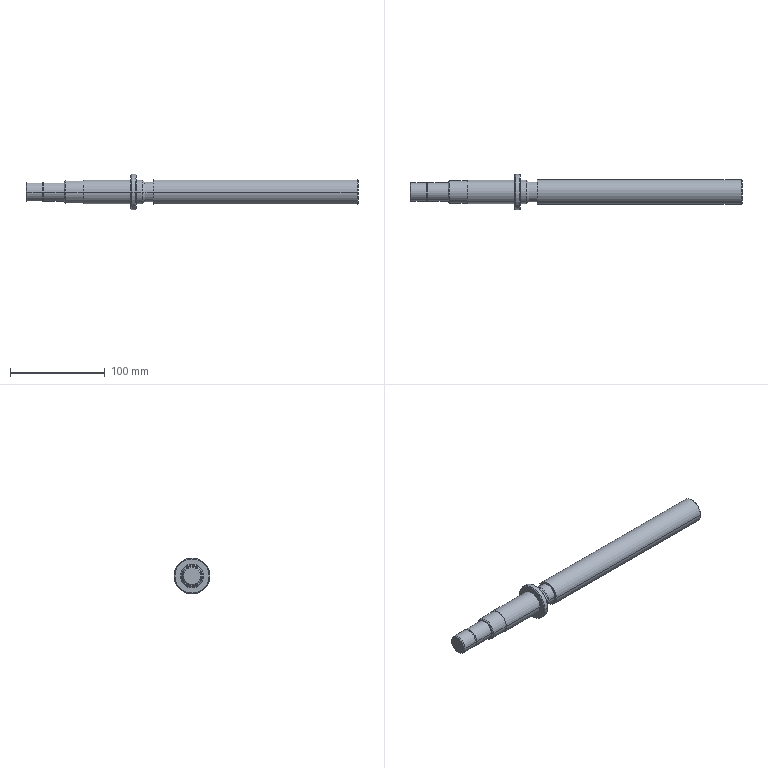Part | SolidWorks | features Chamfer 1, ICE 1, Revolution 1 | 1 solid | 44 faces | box 350.5 x 38 x 38 mm | volume 174413 mm3 | cylinder 20 | cone 12 | plane 12 | commonest cylinder face diameters 20 x4 25 x4 6 x2 18.5 x2 21 x2 24 x2
STEP:
#1=CARTESIAN_POINT('',(0.,-9.,0.));
#2=VERTEX_POINT('',#1);
#3=CARTESIAN_POINT('',(0.,9.,0.));
#4=VERTEX_POINT('',#3);
#5=CARTESIAN_POINT('',(0.,0.,0.));
#6=DIRECTION('',(-1.,0.,0.));
#7=DIRECTION('',(0.,-1.,0.));
#8=AXIS2_PLACEMENT_3D('',#5,#6,#7);
#9=CIRCLE('',#8,9.);
#10=EDGE_CURVE('',#2,#4,#9,.T.);
#11=ORIENTED_EDGE('',*,*,#10,.F.);
#12=CARTESIAN_POINT('',(1.,-10.,0.));
#13=VERTEX_POINT('',#12);
#14=CARTESIAN_POINT('',(1.,-10.,0.));
#15=DIRECTION('',(0.7071,-0.7071,0.));
#16=VECTOR('',#15,1000.);
#17=LINE('',#14,#16);
#18=EDGE_CURVE('',#2,#13,#17,.T.);
#19=ORIENTED_EDGE('',*,*,#18,.T.);
#20=CARTESIAN_POINT('',(1.,10.,0.));
#21=VERTEX_POINT('',#20);
#22=CARTESIAN_POINT('',(1.,0.,0.));
#23=DIRECTION('',(1.,0.,0.));
#24=DIRECTION('',(0.,-1.,0.));
#25=AXIS2_PLACEMENT_3D('',#22,#23,#24);
#26=CIRCLE('',#25,10.);
#27=EDGE_CURVE('',#21,#13,#26,.T.);
#28=ORIENTED_EDGE('',*,*,#27,.F.);
#29=CARTESIAN_POINT('',(1.,10.,0.));
#30=DIRECTION('',(0.7071,0.7071,0.));
#31=VECTOR('',#30,1000.);
#32=LINE('',#29,#31);
#33=EDGE_CURVE('',#4,#21,#32,.T.);
#34=ORIENTED_EDGE('',*,*,#33,.F.);
#35=EDGE_LOOP('',(#11,#19,#28,#34));
#36=FACE_OUTER_BOUND('',#35,.T.);
#37=CARTESIAN_POINT('',(1.,0.,0.));
#38=DIRECTION('',(1.,0.,0.));
#39=DIRECTION('',(0.,1.,0.));
#40=AXIS2_PLACEMENT_3D('',#37,#38,#39);
#41=CONICAL_SURFACE('',#40,10.,0.7854);
#42=ADVANCED_FACE('',(#36),#41,.T.);
#43=CARTESIAN_POINT('',(40.5,-11.,0.));
#44=VERTEX_POINT('',#43);
#45=CARTESIAN_POINT('',(40.5,11.,0.));
#46=VERTEX_POINT('',#45);
#47=CARTESIAN_POINT('',(40.5,0.,0.));
#48=DIRECTION('',(-1.,0.,0.));
#49=DIRECTION('',(0.,-1.,0.));
#50=AXIS2_PLACEMENT_3D('',#47,#48,#49);
#51=CIRCLE('',#50,11.);
#52=EDGE_CURVE('',#44,#46,#51,.T.);
#53=ORIENTED_EDGE('',*,*,#52,.F.);
#54=CARTESIAN_POINT('',(41.5,-12.,0.));
#55=VERTEX_POINT('',#54);
#56=CARTESIAN_POINT('',(41.5,-12.,0.));
#57=DIRECTION('',(0.7071,-0.7071,0.));
#58=VECTOR('',#57,1000.);
#59=LINE('',#56,#58);
#60=EDGE_CURVE('',#44,#55,#59,.T.);
#61=ORIENTED_EDGE('',*,*,#60,.T.);
#62=CARTESIAN_POINT('',(41.5,12.,0.));
#63=VERTEX_POINT('',#62);
#64=CARTESIAN_POINT('',(41.5,0.,0.));
#65=DIRECTION('',(1.,0.,0.));
#66=DIRECTION('',(0.,-1.,0.));
#67=AXIS2_PLACEMENT_3D('',#64,#65,#66);
#68=CIRCLE('',#67,12.);
#69=EDGE_CURVE('',#63,#55,#68,.T.);
#70=ORIENTED_EDGE('',*,*,#69,.F.);
#71=CARTESIAN_POINT('',(41.5,12.,0.));
#72=DIRECTION('',(0.7071,0.7071,0.));
#73=VECTOR('',#72,1000.);
#74=LINE('',#71,#73);
#75=EDGE_CURVE('',#46,#63,#74,.T.);
#76=ORIENTED_EDGE('',*,*,#75,.F.);
#77=EDGE_LOOP('',(#53,#61,#70,#76));
#78=FACE_OUTER_BOUND('',#77,.T.);
#79=CARTESIAN_POINT('',(41.5,0.,0.));
#80=DIRECTION('',(1.,0.,0.));
#81=DIRECTION('',(0.,1.,0.));
#82=AXIS2_PLACEMENT_3D('',#79,#80,#81);
#83=CONICAL_SURFACE('',#82,12.,0.7854);
#84=ADVANCED_FACE('',(#78),#83,.T.);
#85=CARTESIAN_POINT('',(110.5,-18.,0.));
#86=VERTEX_POINT('',#85);
#87=CARTESIAN_POINT('',(110.5,18.,0.));
#88=VERTEX_POINT('',#87);
#89=CARTESIAN_POINT('',(110.5,0.,0.));
#90=DIRECTION('',(-1.,0.,0.));
#91=DIRECTION('',(0.,-1.,0.));
#92=AXIS2_PLACEMENT_3D('',#89,#90,#91);
#93=CIRCLE('',#92,18.);
#94=EDGE_CURVE('',#86,#88,#93,.T.);
#95=ORIENTED_EDGE('',*,*,#94,.F.);
#96=CARTESIAN_POINT('',(111.5,-19.,0.));
#97=VERTEX_POINT('',#96);
#98=CARTESIAN_POINT('',(111.5,-19.,0.));
#99=DIRECTION('',(0.7071,-0.7071,0.));
#100=VECTOR('',#99,1000.);
#101=LINE('',#98,#100);
#102=EDGE_CURVE('',#86,#97,#101,.T.);
#103=ORIENTED_EDGE('',*,*,#102,.T.);
#104=CARTESIAN_POINT('',(111.5,19.,0.));
#105=VERTEX_POINT('',#104);
#106=CARTESIAN_POINT('',(111.5,0.,0.));
#107=DIRECTION('',(1.,0.,0.));
#108=DIRECTION('',(0.,-1.,0.));
#109=AXIS2_PLACEMENT_3D('',#106,#107,#108);
#110=CIRCLE('',#109,19.);
#111=EDGE_CURVE('',#105,#97,#110,.T.);
#112=ORIENTED_EDGE('',*,*,#111,.F.);
#113=CARTESIAN_POINT('',(111.5,19.,0.));
#114=DIRECTION('',(0.7071,0.7071,0.));
#115=VECTOR('',#114,1000.);
#116=LINE('',#113,#115);
#117=EDGE_CURVE('',#88,#105,#116,.T.);
#118=ORIENTED_EDGE('',*,*,#117,.F.);
#119=EDGE_LOOP('',(#95,#103,#112,#118));
#120=FACE_OUTER_BOUND('',#119,.T.);
#121=CARTESIAN_POINT('',(111.5,0.,0.));
#122=DIRECTION('',(1.,0.,0.));
#123=DIRECTION('',(0.,1.,0.));
#124=AXIS2_PLACEMENT_3D('',#121,#122,#123);
#125=CONICAL_SURFACE('',#124,19.,0.7854);
#126=ADVANCED_FACE('',(#120),#125,.T.);
#127=CARTESIAN_POINT('',(116.5,18.,0.));
#128=VERTEX_POINT('',#127);
#129=CARTESIAN_POINT('',(116.5,-18.,0.));
#130=VERTEX_POINT('',#129);
#131=CARTESIAN_POINT('',(116.5,0.,0.));
#132=DIRECTION('',(1.,0.,0.));
#133=DIRECTION('',(0.,1.,0.));
#134=AXIS2_PLACEMENT_3D('',#131,#132,#133);
#135=CIRCLE('',#134,18.);
#136=EDGE_CURVE('',#128,#130,#135,.T.);
#137=ORIENTED_EDGE('',*,*,#136,.F.);
#138=CARTESIAN_POINT('',(115.5,19.,0.));
#139=VERTEX_POINT('',#138);
#140=CARTESIAN_POINT('',(116.5,18.,0.));
#141=DIRECTION('',(-0.7071,0.7071,0.));
#142=VECTOR('',#141,1000.);
#143=LINE('',#140,#142);
#144=EDGE_CURVE('',#128,#139,#143,.T.);
#145=ORIENTED_EDGE('',*,*,#144,.T.);
#146=CARTESIAN_POINT('',(115.5,-19.,0.));
#147=VERTEX_POINT('',#146);
#148=CARTESIAN_POINT('',(115.5,0.,0.));
#149=DIRECTION('',(-1.,0.,0.));
#150=DIRECTION('',(0.,1.,0.));
#151=AXIS2_PLACEMENT_3D('',#148,#149,#150);
#152=CIRCLE('',#151,19.);
#153=EDGE_CURVE('',#147,#139,#152,.T.);
#154=ORIENTED_EDGE('',*,*,#153,.F.);
#155=CARTESIAN_POINT('',(116.5,-18.,0.));
#156=DIRECTION('',(-0.7071,-0.7071,0.));
#157=VECTOR('',#156,1000.);
#158=LINE('',#155,#157);
#159=EDGE_CURVE('',#130,#147,#158,.T.);
#160=ORIENTED_EDGE('',*,*,#159,.F.);
#161=EDGE_LOOP('',(#137,#145,#154,#160));
#162=FACE_OUTER_BOUND('',#161,.T.);
#163=CARTESIAN_POINT('',(116.5,0.,0.));
#164=DIRECTION('',(-1.,0.,0.));
#165=DIRECTION('',(0.,-1.,0.));
#166=AXIS2_PLACEMENT_3D('',#163,#164,#165);
#167=CONICAL_SURFACE('',#166,18.,0.7854);
#168=ADVANCED_FACE('',(#162),#167,.T.);
#169=CARTESIAN_POINT('',(350.5,12.,0.));
#170=VERTEX_POINT('',#169);
#171=CARTESIAN_POINT('',(350.5,-12.,0.));
#172=VERTEX_POINT('',#171);
#173=CARTESIAN_POINT('',(350.5,0.,0.));
#174=DIRECTION('',(1.,0.,0.));
#175=DIRECTION('',(0.,1.,0.));
#176=AXIS2_PLACEMENT_3D('',#173,#174,#175);
#177=CIRCLE('',#176,12.);
#178=EDGE_CURVE('',#170,#172,#177,.T.);
#179=ORIENTED_EDGE('',*,*,#178,.F.);
#180=CARTESIAN_POINT('',(349.5,13.,0.));
#181=VERTEX_POINT('',#180);
#182=CARTESIAN_POINT('',(350.5,12.,0.));
#183=DIRECTION('',(-0.7071,0.7071,0.));
#184=VECTOR('',#183,1000.);
#185=LINE('',#182,#184);
#186=EDGE_CURVE('',#170,#181,#185,.T.);
#187=ORIENTED_EDGE('',*,*,#186,.T.);
#188=CARTESIAN_POINT('',(349.5,-13.,0.));
#189=VERTEX_POINT('',#188);
#190=CARTESIAN_POINT('',(349.5,0.,0.));
#191=DIRECTION('',(-1.,0.,0.));
#192=DIRECTION('',(0.,1.,0.));
#193=AXIS2_PLACEMENT_3D('',#190,#191,#192);
#194=CIRCLE('',#193,13.);
#195=EDGE_CURVE('',#189,#181,#194,.T.);
#196=ORIENTED_EDGE('',*,*,#195,.F.);
#197=CARTESIAN_POINT('',(350.5,-12.,0.));
#198=DIRECTION('',(-0.7071,-0.7071,0.));
#199=VECTOR('',#198,1000.);
#200=LINE('',#197,#199);
#201=EDGE_CURVE('',#172,#189,#200,.T.);
#202=ORIENTED_EDGE('',*,*,#201,.F.);
#203=EDGE_LOOP('',(#179,#187,#196,#202));
#204=FACE_OUTER_BOUND('',#203,.T.);
#205=CARTESIAN_POINT('',(350.5,0.,0.));
#206=DIRECTION('',(-1.,0.,0.));
#207=DIRECTION('',(0.,-1.,0.));
#208=AXIS2_PLACEMENT_3D('',#205,#206,#207);
#209=CONICAL_SURFACE('',#208,12.,0.7854);
#210=ADVANCED_FACE('',(#204),#209,.T.);
#211=CARTESIAN_POINT('',(134.5,13.,0.));
#212=VERTEX_POINT('',#211);
#213=CARTESIAN_POINT('',(134.5,-13.,0.));
#214=VERTEX_POINT('',#213);
#215=CARTESIAN_POINT('',(134.5,0.,0.));
#216=DIRECTION('',(1.,0.,0.));
#217=DIRECTION('',(0.,1.,0.));
#218=AXIS2_PLACEMENT_3D('',#215,#216,#217);
#219=CIRCLE('',#218,13.);
#220=EDGE_CURVE('',#212,#214,#219,.T.);
#221=ORIENTED_EDGE('',*,*,#220,.T.);
#222=CARTESIAN_POINT('',(350.5,-13.,0.));
#223=DIRECTION('',(1.,0.,0.));
#224=VECTOR('',#223,1000.);
#225=LINE('',#222,#224);
#226=EDGE_CURVE('',#214,#189,#225,.T.);
#227=ORIENTED_EDGE('',*,*,#226,.T.);
#228=ORIENTED_EDGE('',*,*,#195,.T.);
#229=CARTESIAN_POINT('',(350.5,13.,0.));
#230=DIRECTION('',(1.,0.,0.));
#231=VECTOR('',#230,1000.);
#232=LINE('',#229,#231);
#233=EDGE_CURVE('',#212,#181,#232,.T.);
#234=ORIENTED_EDGE('',*,*,#233,.F.);
#235=EDGE_LOOP('',(#221,#227,#228,#234));
#236=FACE_OUTER_BOUND('',#235,.T.);
#237=CARTESIAN_POINT('',(350.5,0.,0.));
#238=DIRECTION('',(1.,0.,0.));
#239=DIRECTION('',(0.,1.,0.));
#240=AXIS2_PLACEMENT_3D('',#237,#238,#239);
#241=CYLINDRICAL_SURFACE('',#240,13.);
#242=ADVANCED_FACE('',(#236),#241,.T.);
#243=CARTESIAN_POINT('',(125.5,10.5,0.));
#244=VERTEX_POINT('',#243);
#245=CARTESIAN_POINT('',(125.5,-10.5,0.));
#246=VERTEX_POINT('',#245);
#247=CARTESIAN_POINT('',(125.5,0.,0.));
#248=DIRECTION('',(1.,0.,0.));
#249=DIRECTION('',(0.,1.,0.));
#250=AXIS2_PLACEMENT_3D('',#247,#248,#249);
#251=CIRCLE('',#250,10.5);
#252=EDGE_CURVE('',#244,#246,#251,.T.);
#253=ORIENTED_EDGE('',*,*,#252,.T.);
#254=CARTESIAN_POINT('',(134.5,-10.5,0.));
#255=VERTEX_POINT('',#254);
#256=CARTESIAN_POINT('',(350.5,-10.5,0.));
#257=DIRECTION('',(1.,0.,0.));
#258=VECTOR('',#257,1000.);
#259=LINE('',#256,#258);
#260=EDGE_CURVE('',#246,#255,#259,.T.);
#261=ORIENTED_EDGE('',*,*,#260,.T.);
#262=CARTESIAN_POINT('',(134.5,10.5,0.));
#263=VERTEX_POINT('',#262);
#264=CARTESIAN_POINT('',(134.5,0.,0.));
#265=DIRECTION('',(1.,0.,0.));
#266=DIRECTION('',(0.,1.,0.));
#267=AXIS2_PLACEMENT_3D('',#264,#265,#266);
#268=CIRCLE('',#267,10.5);
#269=EDGE_CURVE('',#263,#255,#268,.T.);
#270=ORIENTED_EDGE('',*,*,#269,.F.);
#271=CARTESIAN_POINT('',(350.5,10.5,0.));
#272=DIRECTION('',(1.,0.,0.));
#273=VECTOR('',#272,1000.);
#274=LINE('',#271,#273);
#275=EDGE_CURVE('',#244,#263,#274,.T.);
#276=ORIENTED_EDGE('',*,*,#275,.F.);
#277=EDGE_LOOP('',(#253,#261,#270,#276));
#278=FACE_OUTER_BOUND('',#277,.T.);
#279=CARTESIAN_POINT('',(350.5,0.,0.));
#280=DIRECTION('',(1.,0.,0.));
#281=DIRECTION('',(0.,1.,0.));
#282=AXIS2_PLACEMENT_3D('',#279,#280,#281);
#283=CYLINDRICAL_SURFACE('',#282,10.5);
#284=ADVANCED_FACE('',(#278),#283,.T.);
#285=ORIENTED_EDGE('',*,*,#252,.F.);
#286=CARTESIAN_POINT('',(122.5,12.5,0.));
#287=VERTEX_POINT('',#286);
#288=CARTESIAN_POINT('',(125.5,10.5,0.));
#289=DIRECTION('',(-0.8321,0.5547,0.));
#290=VECTOR('',#289,1000.);
#291=LINE('',#288,#290);
#292=EDGE_CURVE('',#244,#287,#291,.T.);
#293=ORIENTED_EDGE('',*,*,#292,.T.);
#294=CARTESIAN_POINT('',(122.5,-12.5,0.));
#295=VERTEX_POINT('',#294);
#296=CARTESIAN_POINT('',(122.5,0.,0.));
#297=DIRECTION('',(1.,0.,0.));
#298=DIRECTION('',(0.,1.,0.));
#299=AXIS2_PLACEMENT_3D('',#296,#297,#298);
#300=CIRCLE('',#299,12.5);
#301=EDGE_CURVE('',#287,#295,#300,.T.);
#302=ORIENTED_EDGE('',*,*,#301,.T.);
#303=CARTESIAN_POINT('',(125.5,-10.5,0.));
#304=DIRECTION('',(-0.8321,-0.5547,0.));
#305=VECTOR('',#304,1000.);
#306=LINE('',#303,#305);
#307=EDGE_CURVE('',#246,#295,#306,.T.);
#308=ORIENTED_EDGE('',*,*,#307,.F.);
#309=EDGE_LOOP('',(#285,#293,#302,#308));
#310=FACE_OUTER_BOUND('',#309,.T.);
#311=CARTESIAN_POINT('',(125.5,0.,0.));
#312=DIRECTION('',(-1.,0.,0.));
#313=DIRECTION('',(0.,-1.,0.));
#314=AXIS2_PLACEMENT_3D('',#311,#312,#313);
#315=CONICAL_SURFACE('',#314,10.5,0.588);
#316=ADVANCED_FACE('',(#310),#315,.T.);
#317=CARTESIAN_POINT('',(116.5,12.5,0.));
#318=VERTEX_POINT('',#317);
#319=CARTESIAN_POINT('',(116.5,-12.5,0.));
#320=VERTEX_POINT('',#319);
#321=CARTESIAN_POINT('',(116.5,0.,0.));
#322=DIRECTION('',(1.,0.,0.));
#323=DIRECTION('',(0.,1.,0.));
#324=AXIS2_PLACEMENT_3D('',#321,#322,#323);
#325=CIRCLE('',#324,12.5);
#326=EDGE_CURVE('',#318,#320,#325,.T.);
#327=ORIENTED_EDGE('',*,*,#326,.T.);
#328=CARTESIAN_POINT('',(350.5,-12.5,0.));
#329=DIRECTION('',(1.,0.,0.));
#330=VECTOR('',#329,1000.);
#331=LINE('',#328,#330);
#332=EDGE_CURVE('',#320,#295,#331,.T.);
#333=ORIENTED_EDGE('',*,*,#332,.T.);
#334=ORIENTED_EDGE('',*,*,#301,.F.);
#335=CARTESIAN_POINT('',(350.5,12.5,0.));
#336=DIRECTION('',(1.,0.,0.));
#337=VECTOR('',#336,1000.);
#338=LINE('',#335,#337);
#339=EDGE_CURVE('',#318,#287,#338,.T.);
#340=ORIENTED_EDGE('',*,*,#339,.F.);
#341=EDGE_LOOP('',(#327,#333,#334,#340));
#342=FACE_OUTER_BOUND('',#341,.T.);
#343=CARTESIAN_POINT('',(350.5,0.,0.));
#344=DIRECTION('',(1.,0.,0.));
#345=DIRECTION('',(0.,1.,0.));
#346=AXIS2_PLACEMENT_3D('',#343,#344,#345);
#347=CYLINDRICAL_SURFACE('',#346,12.5);
#348=ADVANCED_FACE('',(#342),#347,.T.);
#349=ORIENTED_EDGE('',*,*,#111,.T.);
#350=CARTESIAN_POINT('',(350.5,-19.,0.));
#351=DIRECTION('',(1.,0.,0.));
#352=VECTOR('',#351,1000.);
#353=LINE('',#350,#352);
#354=EDGE_CURVE('',#97,#147,#353,.T.);
#355=ORIENTED_EDGE('',*,*,#354,.T.);
#356=ORIENTED_EDGE('',*,*,#153,.T.);
#357=CARTESIAN_POINT('',(350.5,19.,0.));
#358=DIRECTION('',(1.,0.,0.));
#359=VECTOR('',#358,1000.);
#360=LINE('',#357,#359);
#361=EDGE_CURVE('',#105,#139,#360,.T.);
#362=ORIENTED_EDGE('',*,*,#361,.F.);
#363=EDGE_LOOP('',(#349,#355,#356,#362));
#364=FACE_OUTER_BOUND('',#363,.T.);
#365=CARTESIAN_POINT('',(350.5,0.,0.));
#366=DIRECTION('',(1.,0.,0.));
#367=DIRECTION('',(0.,1.,0.));
#368=AXIS2_PLACEMENT_3D('',#365,#366,#367);
#369=CYLINDRICAL_SURFACE('',#368,19.);
#370=ADVANCED_FACE('',(#364),#369,.T.);
#371=CARTESIAN_POINT('',(60.5,12.5,0.));
#372=VERTEX_POINT('',#371);
#373=CARTESIAN_POINT('',(60.5,-12.5,0.));
#374=VERTEX_POINT('',#373);
#375=CARTESIAN_POINT('',(60.5,0.,0.));
#376=DIRECTION('',(1.,0.,0.));
#377=DIRECTION('',(0.,1.,0.));
#378=AXIS2_PLACEMENT_3D('',#375,#376,#377);
#379=CIRCLE('',#378,12.5);
#380=EDGE_CURVE('',#372,#374,#379,.T.);
#381=ORIENTED_EDGE('',*,*,#380,.T.);
#382=CARTESIAN_POINT('',(110.5,-12.5,0.));
#383=VERTEX_POINT('',#382);
#384=CARTESIAN_POINT('',(350.5,-12.5,0.));
#385=DIRECTION('',(1.,0.,0.));
#386=VECTOR('',#385,1000.);
#387=LINE('',#384,#386);
#388=EDGE_CURVE('',#374,#383,#387,.T.);
#389=ORIENTED_EDGE('',*,*,#388,.T.);
#390=CARTESIAN_POINT('',(110.5,12.5,0.));
#391=VERTEX_POINT('',#390);
#392=CARTESIAN_POINT('',(110.5,0.,0.));
#393=DIRECTION('',(1.,0.,0.));
#394=DIRECTION('',(0.,1.,0.));
#395=AXIS2_PLACEMENT_3D('',#392,#393,#394);
#396=CIRCLE('',#395,12.5);
#397=EDGE_CURVE('',#391,#383,#396,.T.);
#398=ORIENTED_EDGE('',*,*,#397,.F.);
#399=CARTESIAN_POINT('',(350.5,12.5,0.));
#400=DIRECTION('',(1.,0.,0.));
#401=VECTOR('',#400,1000.);
#402=LINE('',#399,#401);
#403=EDGE_CURVE('',#372,#391,#402,.T.);
#404=ORIENTED_EDGE('',*,*,#403,.F.);
#405=EDGE_LOOP('',(#381,#389,#398,#404));
#406=FACE_OUTER_BOUND('',#405,.T.);
#407=CARTESIAN_POINT('',(350.5,0.,0.));
#408=DIRECTION('',(1.,0.,0.));
#409=DIRECTION('',(0.,1.,0.));
#410=AXIS2_PLACEMENT_3D('',#407,#408,#409);
#411=CYLINDRICAL_SURFACE('',#410,12.5);
#412=ADVANCED_FACE('',(#406),#411,.T.);
#413=ORIENTED_EDGE('',*,*,#69,.T.);
#414=CARTESIAN_POINT('',(60.5,-12.,0.));
#415=VERTEX_POINT('',#414);
#416=CARTESIAN_POINT('',(350.5,-12.,0.));
#417=DIRECTION('',(1.,0.,0.));
#418=VECTOR('',#417,1000.);
#419=LINE('',#416,#418);
#420=EDGE_CURVE('',#55,#415,#419,.T.);
#421=ORIENTED_EDGE('',*,*,#420,.T.);
#422=CARTESIAN_POINT('',(60.5,12.,0.));
#423=VERTEX_POINT('',#422);
#424=CARTESIAN_POINT('',(60.5,0.,0.));
#425=DIRECTION('',(1.,0.,0.));
#426=DIRECTION('',(0.,1.,0.));
#427=AXIS2_PLACEMENT_3D('',#424,#425,#426);
#428=CIRCLE('',#427,12.);
#429=EDGE_CURVE('',#423,#415,#428,.T.);
#430=ORIENTED_EDGE('',*,*,#429,.F.);
#431=CARTESIAN_POINT('',(350.5,12.,0.));
#432=DIRECTION('',(1.,0.,0.));
#433=VECTOR('',#432,1000.);
#434=LINE('',#431,#433);
#435=EDGE_CURVE('',#63,#423,#434,.T.);
#436=ORIENTED_EDGE('',*,*,#435,.F.);
#437=EDGE_LOOP('',(#413,#421,#430,#436));
#438=FACE_OUTER_BOUND('',#437,.T.);
#439=CARTESIAN_POINT('',(350.5,0.,0.));
#440=DIRECTION('',(1.,0.,0.));
#441=DIRECTION('',(0.,1.,0.));
#442=AXIS2_PLACEMENT_3D('',#439,#440,#441);
#443=CYLINDRICAL_SURFACE('',#442,12.);
#444=ADVANCED_FACE('',(#438),#443,.T.);
#445=CARTESIAN_POINT('',(17.,9.25,0.));
#446=VERTEX_POINT('',#445);
#447=CARTESIAN_POINT('',(17.,-9.25,0.));
#448=VERTEX_POINT('',#447);
#449=CARTESIAN_POINT('',(17.,0.,0.));
#450=DIRECTION('',(1.,0.,0.));
#451=DIRECTION('',(0.,1.,0.));
#452=AXIS2_PLACEMENT_3D('',#449,#450,#451);
#453=CIRCLE('',#452,9.25);
#454=EDGE_CURVE('',#446,#448,#453,.T.);
#455=ORIENTED_EDGE('',*,*,#454,.T.);
#456=CARTESIAN_POINT('',(18.5,-9.25,0.));
#457=VERTEX_POINT('',#456);
#458=CARTESIAN_POINT('',(350.5,-9.25,0.));
#459=DIRECTION('',(1.,0.,0.));
#460=VECTOR('',#459,1000.);
#461=LINE('',#458,#460);
#462=EDGE_CURVE('',#448,#457,#461,.T.);
#463=ORIENTED_EDGE('',*,*,#462,.T.);
#464=CARTESIAN_POINT('',(18.5,9.25,0.));
#465=VERTEX_POINT('',#464);
#466=CARTESIAN_POINT('',(18.5,0.,0.));
#467=DIRECTION('',(1.,0.,0.));
#468=DIRECTION('',(0.,1.,0.));
#469=AXIS2_PLACEMENT_3D('',#466,#467,#468);
#470=CIRCLE('',#469,9.25);
#471=EDGE_CURVE('',#465,#457,#470,.T.);
#472=ORIENTED_EDGE('',*,*,#471,.F.);
#473=CARTESIAN_POINT('',(350.5,9.25,0.));
#474=DIRECTION('',(1.,0.,0.));
#475=VECTOR('',#474,1000.);
#476=LINE('',#473,#475);
#477=EDGE_CURVE('',#446,#465,#476,.T.);
#478=ORIENTED_EDGE('',*,*,#477,.F.);
#479=EDGE_LOOP('',(#455,#463,#472,#478));
#480=FACE_OUTER_BOUND('',#479,.T.);
#481=CARTESIAN_POINT('',(350.5,0.,0.));
#482=DIRECTION('',(1.,0.,0.));
#483=DIRECTION('',(0.,1.,0.));
#484=AXIS2_PLACEMENT_3D('',#481,#482,#483);
#485=CYLINDRICAL_SURFACE('',#484,9.25);
#486=ADVANCED_FACE('',(#480),#485,.T.);
#487=ORIENTED_EDGE('',*,*,#27,.T.);
#488=CARTESIAN_POINT('',(17.,-10.,0.));
#489=VERTEX_POINT('',#488);
#490=CARTESIAN_POINT('',(350.5,-10.,0.));
#491=DIRECTION('',(1.,0.,0.));
#492=VECTOR('',#491,1000.);
#493=LINE('',#490,#492);
#494=EDGE_CURVE('',#13,#489,#493,.T.);
#495=ORIENTED_EDGE('',*,*,#494,.T.);
#496=CARTESIAN_POINT('',(17.,10.,0.));
#497=VERTEX_POINT('',#496);
#498=CARTESIAN_POINT('',(17.,0.,0.));
#499=DIRECTION('',(1.,0.,0.));
#500=DIRECTION('',(0.,1.,0.));
#501=AXIS2_PLACEMENT_3D('',#498,#499,#500);
#502=CIRCLE('',#501,10.);
#503=EDGE_CURVE('',#497,#489,#502,.T.);
#504=ORIENTED_EDGE('',*,*,#503,.F.);
#505=CARTESIAN_POINT('',(350.5,10.,0.));
#506=DIRECTION('',(1.,0.,0.));
#507=VECTOR('',#506,1000.);
#508=LINE('',#505,#507);
#509=EDGE_CURVE('',#21,#497,#508,.T.);
#510=ORIENTED_EDGE('',*,*,#509,.F.);
#511=EDGE_LOOP('',(#487,#495,#504,#510));
#512=FACE_OUTER_BOUND('',#511,.T.);
#513=CARTESIAN_POINT('',(350.5,0.,0.));
#514=DIRECTION('',(1.,0.,0.));
#515=DIRECTION('',(0.,1.,0.));
#516=AXIS2_PLACEMENT_3D('',#513,#514,#515);
#517=CYLINDRICAL_SURFACE('',#516,10.);
#518=ADVANCED_FACE('',(#512),#517,.T.);
#519=CARTESIAN_POINT('',(18.5,10.,0.));
#520=VERTEX_POINT('',#519);
#521=CARTESIAN_POINT('',(18.5,-10.,0.));
#522=VERTEX_POINT('',#521);
#523=CARTESIAN_POINT('',(18.5,0.,0.));
#524=DIRECTION('',(1.,0.,0.));
#525=DIRECTION('',(0.,1.,0.));
#526=AXIS2_PLACEMENT_3D('',#523,#524,#525);
#527=CIRCLE('',#526,10.);
#528=EDGE_CURVE('',#520,#522,#527,.T.);
#529=ORIENTED_EDGE('',*,*,#528,.T.);
#530=CARTESIAN_POINT('',(40.5,-10.,0.));
#531=VERTEX_POINT('',#530);
#532=CARTESIAN_POINT('',(350.5,-10.,0.));
#533=DIRECTION('',(1.,0.,0.));
#534=VECTOR('',#533,1000.);
#535=LINE('',#532,#534);
#536=EDGE_CURVE('',#522,#531,#535,.T.);
#537=ORIENTED_EDGE('',*,*,#536,.T.);
#538=CARTESIAN_POINT('',(40.5,10.,0.));
#539=VERTEX_POINT('',#538);
#540=CARTESIAN_POINT('',(40.5,0.,0.));
#541=DIRECTION('',(1.,0.,0.));
#542=DIRECTION('',(0.,1.,0.));
#543=AXIS2_PLACEMENT_3D('',#540,#541,#542);
#544=CIRCLE('',#543,10.);
#545=EDGE_CURVE('',#539,#531,#544,.T.);
#546=ORIENTED_EDGE('',*,*,#545,.F.);
#547=CARTESIAN_POINT('',(37.5,9.539,3.));
#548=VERTEX_POINT('',#547);
#549=CARTESIAN_POINT('',(40.5,10.,0.));
#550=CARTESIAN_POINT('',(40.5,10.,0.1993));
#551=CARTESIAN_POINT('',(40.48,9.994,0.3951));
#552=CARTESIAN_POINT('',(40.403,9.971,0.7799));
#553=CARTESIAN_POINT('',(40.345,9.954,0.971));
#554=CARTESIAN_POINT('',(40.194,9.912,1.334));
#555=CARTESIAN_POINT('',(40.102,9.887,1.505));
#556=CARTESIAN_POINT('',(39.885,9.832,1.831));
#557=CARTESIAN_POINT('',(39.759,9.802,1.984));
#558=CARTESIAN_POINT('',(39.347,9.713,2.396));
#559=CARTESIAN_POINT('',(39.014,9.652,2.619));
#560=CARTESIAN_POINT('',(38.474,9.587,2.844));
#561=CARTESIAN_POINT('',(38.284,9.57,2.902));
#562=CARTESIAN_POINT('',(37.896,9.546,2.98));
#563=CARTESIAN_POINT('',(37.699,9.539,3.));
#564=CARTESIAN_POINT('',(37.5,9.539,3.));
#565=B_SPLINE_CURVE_WITH_KNOTS('',3,(#549,#550,#551,#552,#553,#554,#555,#556,#557,#558,#559,#560,#561,#562,#563,#564),.UNSPECIFIED.,.F.,.F.,(4,2,2,2,2,2,2,4),(0.,0.0005892,0.001178,0.001768,0.002357,0.003535,0.004125,0.004714),.UNSPECIFIED.);
#566=EDGE_CURVE('',#539,#548,#565,.T.);
#567=ORIENTED_EDGE('',*,*,#566,.T.);
#568=CARTESIAN_POINT('',(22.,9.539,3.));
#569=VERTEX_POINT('',#568);
#570=CARTESIAN_POINT('',(350.5,9.539,3.));
#571=DIRECTION('',(-1.,0.,0.));
#572=VECTOR('',#571,1000.);
#573=LINE('',#570,#572);
#574=EDGE_CURVE('',#548,#569,#573,.T.);
#575=ORIENTED_EDGE('',*,*,#574,.T.);
#576=CARTESIAN_POINT('',(19.,10.,0.));
#577=VERTEX_POINT('',#576);
#578=CARTESIAN_POINT('',(22.,9.539,3.));
#579=CARTESIAN_POINT('',(21.8,9.539,3.));
#580=CARTESIAN_POINT('',(21.605,9.546,2.98));
#581=CARTESIAN_POINT('',(21.219,9.569,2.903));
#582=CARTESIAN_POINT('',(21.028,9.587,2.845));
#583=CARTESIAN_POINT('',(20.665,9.631,2.694));
#584=CARTESIAN_POINT('',(20.494,9.656,2.602));
#585=CARTESIAN_POINT('',(20.168,9.712,2.384));
#586=CARTESIAN_POINT('',(20.015,9.743,2.258));
#587=CARTESIAN_POINT('',(19.603,9.832,1.845));
#588=CARTESIAN_POINT('',(19.38,9.892,1.512));
#589=CARTESIAN_POINT('',(19.155,9.954,0.971));
#590=CARTESIAN_POINT('',(19.097,9.971,0.7806));
#591=CARTESIAN_POINT('',(19.019,9.994,0.3926));
#592=CARTESIAN_POINT('',(19.,10.,0.197));
#593=CARTESIAN_POINT('',(19.,10.,0.));
#594=B_SPLINE_CURVE_WITH_KNOTS('',3,(#578,#579,#580,#581,#582,#583,#584,#585,#586,#587,#588,#589,#590,#591,#592,#593),.UNSPECIFIED.,.F.,.F.,(4,2,2,2,2,2,2,4),(0.,0.0005898,0.00118,0.001769,0.002359,0.003539,0.004128,0.004718),.UNSPECIFIED.);
#595=EDGE_CURVE('',#569,#577,#594,.T.);
#596=ORIENTED_EDGE('',*,*,#595,.T.);
#597=CARTESIAN_POINT('',(350.5,10.,0.));
#598=DIRECTION('',(1.,0.,0.));
#599=VECTOR('',#598,1000.);
#600=LINE('',#597,#599);
#601=EDGE_CURVE('',#520,#577,#600,.T.);
#602=ORIENTED_EDGE('',*,*,#601,.F.);
#603=EDGE_LOOP('',(#529,#537,#546,#567,#575,#596,#602));
#604=FACE_OUTER_BOUND('',#603,.T.);
#605=CARTESIAN_POINT('',(350.5,0.,0.));
#606=DIRECTION('',(1.,0.,0.));
#607=DIRECTION('',(0.,1.,0.));
#608=AXIS2_PLACEMENT_3D('',#605,#606,#607);
#609=CYLINDRICAL_SURFACE('',#608,10.);
#610=ADVANCED_FACE('',(#604),#609,.T.);
#611=ORIENTED_EDGE('',*,*,#536,.F.);
#612=CARTESIAN_POINT('',(18.5,0.,0.));
#613=DIRECTION('',(1.,0.,0.));
#614=DIRECTION('',(0.,1.,0.));
#615=AXIS2_PLACEMENT_3D('',#612,#613,#614);
#616=CIRCLE('',#615,10.);
#617=EDGE_CURVE('',#522,#520,#616,.T.);
#618=ORIENTED_EDGE('',*,*,#617,.T.);
#619=ORIENTED_EDGE('',*,*,#601,.T.);
#620=CARTESIAN_POINT('',(22.,9.539,-3.));
#621=VERTEX_POINT('',#620);
#622=CARTESIAN_POINT('',(19.,10.,0.));
#623=CARTESIAN_POINT('',(19.,10.,-0.1968));
#624=CARTESIAN_POINT('',(19.02,9.994,-0.3967));
#625=CARTESIAN_POINT('',(19.097,9.971,-0.7821));
#626=CARTESIAN_POINT('',(19.154,9.955,-0.9695));
#627=CARTESIAN_POINT('',(19.306,9.912,-1.334));
#628=CARTESIAN_POINT('',(19.399,9.887,-1.507));
#629=CARTESIAN_POINT('',(19.616,9.832,-1.831));
#630=CARTESIAN_POINT('',(19.741,9.802,-1.983));
#631=CARTESIAN_POINT('',(20.017,9.742,-2.26));
#632=CARTESIAN_POINT('',(20.167,9.713,-2.383));
#633=CARTESIAN_POINT('',(20.491,9.657,-2.6));
#634=CARTESIAN_POINT('',(20.667,9.63,-2.694));
#635=CARTESIAN_POINT('',(21.028,9.587,-2.845));
#636=CARTESIAN_POINT('',(21.215,9.57,-2.902));
#637=CARTESIAN_POINT('',(21.601,9.546,-2.98));
#638=CARTESIAN_POINT('',(21.801,9.539,-3.));
#639=CARTESIAN_POINT('',(22.,9.539,-3.));
#640=B_SPLINE_CURVE_WITH_KNOTS('',3,(#622,#623,#624,#625,#626,#627,#628,#629,#630,#631,#632,#633,#634,#635,#636,#637,#638,#639),.UNSPECIFIED.,.F.,.F.,(4,2,2,2,2,2,2,2,4),(0.004718,0.005307,0.005896,0.006485,0.007074,0.007663,0.008252,0.008842,0.009431),.UNSPECIFIED.);
#641=EDGE_CURVE('',#577,#621,#640,.T.);
#642=ORIENTED_EDGE('',*,*,#641,.T.);
#643=CARTESIAN_POINT('',(37.5,9.539,-3.));
#644=VERTEX_POINT('',#643);
#645=CARTESIAN_POINT('',(350.5,9.539,-3.));
#646=DIRECTION('',(1.,0.,0.));
#647=VECTOR('',#646,1000.);
#648=LINE('',#645,#647);
#649=EDGE_CURVE('',#621,#644,#648,.T.);
#650=ORIENTED_EDGE('',*,*,#649,.T.);
#651=CARTESIAN_POINT('',(37.5,9.539,-3.));
#652=CARTESIAN_POINT('',(37.699,9.539,-3.));
#653=CARTESIAN_POINT('',(37.895,9.546,-2.98));
#654=CARTESIAN_POINT('',(38.28,9.569,-2.904));
#655=CARTESIAN_POINT('',(38.471,9.587,-2.845));
#656=CARTESIAN_POINT('',(38.833,9.63,-2.695));
#657=CARTESIAN_POINT('',(39.005,9.656,-2.602));
#658=CARTESIAN_POINT('',(39.33,9.712,-2.385));
#659=CARTESIAN_POINT('',(39.483,9.742,-2.259));
#660=CARTESIAN_POINT('',(39.896,9.832,-1.847));
#661=CARTESIAN_POINT('',(40.119,9.891,-1.515));
#662=CARTESIAN_POINT('',(40.344,9.954,-0.9743));
#663=CARTESIAN_POINT('',(40.402,9.971,-0.7845));
#664=CARTESIAN_POINT('',(40.48,9.994,-0.3961));
#665=CARTESIAN_POINT('',(40.5,10.,-0.1993));
#666=CARTESIAN_POINT('',(40.5,10.,0.));
#667=B_SPLINE_CURVE_WITH_KNOTS('',3,(#651,#652,#653,#654,#655,#656,#657,#658,#659,#660,#661,#662,#663,#664,#665,#666),.UNSPECIFIED.,.F.,.F.,(4,2,2,2,2,2,2,4),(0.,0.0005892,0.001178,0.001768,0.002357,0.003535,0.004125,0.004714),.UNSPECIFIED.);
#668=EDGE_CURVE('',#644,#539,#667,.T.);
#669=ORIENTED_EDGE('',*,*,#668,.T.);
#670=CARTESIAN_POINT('',(40.5,0.,0.));
#671=DIRECTION('',(1.,0.,0.));
#672=DIRECTION('',(0.,1.,0.));
#673=AXIS2_PLACEMENT_3D('',#670,#671,#672);
#674=CIRCLE('',#673,10.);
#675=EDGE_CURVE('',#531,#539,#674,.T.);
#676=ORIENTED_EDGE('',*,*,#675,.F.);
#677=EDGE_LOOP('',(#611,#618,#619,#642,#650,#669,#676));
#678=FACE_OUTER_BOUND('',#677,.T.);
#679=CARTESIAN_POINT('',(350.5,0.,0.));
#680=DIRECTION('',(1.,0.,0.));
#681=DIRECTION('',(0.,1.,0.));
#682=AXIS2_PLACEMENT_3D('',#679,#680,#681);
#683=CYLINDRICAL_SURFACE('',#682,10.);
#684=ADVANCED_FACE('',(#678),#683,.T.);
#685=CARTESIAN_POINT('',(0.,0.,0.));
#686=DIRECTION('',(-1.,0.,0.));
#687=DIRECTION('',(0.,-1.,0.));
#688=AXIS2_PLACEMENT_3D('',#685,#686,#687);
#689=CIRCLE('',#688,9.);
#690=EDGE_CURVE('',#4,#2,#689,.T.);
#691=ORIENTED_EDGE('',*,*,#690,.T.);
#692=ORIENTED_EDGE('',*,*,#10,.T.);
#693=EDGE_LOOP('',(#691,#692));
#694=FACE_OUTER_BOUND('',#693,.T.);
#695=CARTESIAN_POINT('',(0.,0.,0.));
#696=DIRECTION('',(-1.,0.,0.));
#697=DIRECTION('',(0.,-1.,0.));
#698=AXIS2_PLACEMENT_3D('',#695,#696,#697);
#699=PLANE('',#698);
#700=ADVANCED_FACE('',(#694),#699,.T.);
#701=ORIENTED_EDGE('',*,*,#494,.F.);
#702=CARTESIAN_POINT('',(1.,0.,0.));
#703=DIRECTION('',(1.,0.,0.));
#704=DIRECTION('',(0.,-1.,0.));
#705=AXIS2_PLACEMENT_3D('',#702,#703,#704);
#706=CIRCLE('',#705,10.);
#707=EDGE_CURVE('',#13,#21,#706,.T.);
#708=ORIENTED_EDGE('',*,*,#707,.T.);
#709=ORIENTED_EDGE('',*,*,#509,.T.);
#710=CARTESIAN_POINT('',(17.,0.,0.));
#711=DIRECTION('',(1.,0.,0.));
#712=DIRECTION('',(0.,1.,0.));
#713=AXIS2_PLACEMENT_3D('',#710,#711,#712);
#714=CIRCLE('',#713,10.);
#715=EDGE_CURVE('',#489,#497,#714,.T.);
#716=ORIENTED_EDGE('',*,*,#715,.F.);
#717=EDGE_LOOP('',(#701,#708,#709,#716));
#718=FACE_OUTER_BOUND('',#717,.T.);
#719=CARTESIAN_POINT('',(350.5,0.,0.));
#720=DIRECTION('',(1.,0.,0.));
#721=DIRECTION('',(0.,1.,0.));
#722=AXIS2_PLACEMENT_3D('',#719,#720,#721);
#723=CYLINDRICAL_SURFACE('',#722,10.);
#724=ADVANCED_FACE('',(#718),#723,.T.);
#725=ORIENTED_EDGE('',*,*,#503,.T.);
#726=ORIENTED_EDGE('',*,*,#715,.T.);
#727=EDGE_LOOP('',(#725,#726));
#728=FACE_OUTER_BOUND('',#727,.T.);
#729=ORIENTED_EDGE('',*,*,#454,.F.);
#730=CARTESIAN_POINT('',(17.,0.,0.));
#731=DIRECTION('',(1.,0.,0.));
#732=DIRECTION('',(0.,1.,0.));
#733=AXIS2_PLACEMENT_3D('',#730,#731,#732);
#734=CIRCLE('',#733,9.25);
#735=EDGE_CURVE('',#448,#446,#734,.T.);
#736=ORIENTED_EDGE('',*,*,#735,.F.);
#737=EDGE_LOOP('',(#729,#736));
#738=FACE_BOUND('',#737,.T.);
#739=CARTESIAN_POINT('',(17.,10.,0.));
#740=DIRECTION('',(1.,0.,0.));
#741=DIRECTION('',(0.,1.,0.));
#742=AXIS2_PLACEMENT_3D('',#739,#740,#741);
#743=PLANE('',#742);
#744=ADVANCED_FACE('',(#728,#738),#743,.T.);
#745=ORIENTED_EDGE('',*,*,#462,.F.);
#746=ORIENTED_EDGE('',*,*,#735,.T.);
#747=ORIENTED_EDGE('',*,*,#477,.T.);
#748=CARTESIAN_POINT('',(18.5,0.,0.));
#749=DIRECTION('',(1.,0.,0.));
#750=DIRECTION('',(0.,1.,0.));
#751=AXIS2_PLACEMENT_3D('',#748,#749,#750);
#752=CIRCLE('',#751,9.25);
#753=EDGE_CURVE('',#457,#465,#752,.T.);
#754=ORIENTED_EDGE('',*,*,#753,.F.);
#755=EDGE_LOOP('',(#745,#746,#747,#754));
#756=FACE_OUTER_BOUND('',#755,.T.);
#757=CARTESIAN_POINT('',(350.5,0.,0.));
#758=DIRECTION('',(1.,0.,0.));
#759=DIRECTION('',(0.,1.,0.));
#760=AXIS2_PLACEMENT_3D('',#757,#758,#759);
#761=CYLINDRICAL_SURFACE('',#760,9.25);
#762=ADVANCED_FACE('',(#756),#761,.T.);
#763=ORIENTED_EDGE('',*,*,#471,.T.);
#764=ORIENTED_EDGE('',*,*,#753,.T.);
#765=EDGE_LOOP('',(#763,#764));
#766=FACE_BOUND('',#765,.T.);
#767=ORIENTED_EDGE('',*,*,#528,.F.);
#768=ORIENTED_EDGE('',*,*,#617,.F.);
#769=EDGE_LOOP('',(#767,#768));
#770=FACE_OUTER_BOUND('',#769,.T.);
#771=CARTESIAN_POINT('',(18.5,9.25,0.));
#772=DIRECTION('',(-1.,0.,0.));
#773=DIRECTION('',(0.,-1.,0.));
#774=AXIS2_PLACEMENT_3D('',#771,#772,#773);
#775=PLANE('',#774);
#776=ADVANCED_FACE('',(#766,#770),#775,.T.);
#777=CARTESIAN_POINT('',(40.5,0.,0.));
#778=DIRECTION('',(-1.,0.,0.));
#779=DIRECTION('',(0.,-1.,0.));
#780=AXIS2_PLACEMENT_3D('',#777,#778,#779);
#781=CIRCLE('',#780,11.);
#782=EDGE_CURVE('',#46,#44,#781,.T.);
#783=ORIENTED_EDGE('',*,*,#782,.T.);
#784=ORIENTED_EDGE('',*,*,#52,.T.);
#785=EDGE_LOOP('',(#783,#784));
#786=FACE_OUTER_BOUND('',#785,.T.);
#787=ORIENTED_EDGE('',*,*,#545,.T.);
#788=ORIENTED_EDGE('',*,*,#675,.T.);
#789=EDGE_LOOP('',(#787,#788));
#790=FACE_BOUND('',#789,.T.);
#791=CARTESIAN_POINT('',(40.5,10.,0.));
#792=DIRECTION('',(-1.,0.,0.));
#793=DIRECTION('',(0.,-1.,0.));
#794=AXIS2_PLACEMENT_3D('',#791,#792,#793);
#795=PLANE('',#794);
#796=ADVANCED_FACE('',(#786,#790),#795,.T.);
#797=ORIENTED_EDGE('',*,*,#420,.F.);
#798=CARTESIAN_POINT('',(41.5,0.,0.));
#799=DIRECTION('',(1.,0.,0.));
#800=DIRECTION('',(0.,-1.,0.));
#801=AXIS2_PLACEMENT_3D('',#798,#799,#800);
#802=CIRCLE('',#801,12.);
#803=EDGE_CURVE('',#55,#63,#802,.T.);
#804=ORIENTED_EDGE('',*,*,#803,.T.);
#805=ORIENTED_EDGE('',*,*,#435,.T.);
#806=CARTESIAN_POINT('',(60.5,0.,0.));
#807=DIRECTION('',(1.,0.,0.));
#808=DIRECTION('',(0.,1.,0.));
#809=AXIS2_PLACEMENT_3D('',#806,#807,#808);
#810=CIRCLE('',#809,12.);
#811=EDGE_CURVE('',#415,#423,#810,.T.);
#812=ORIENTED_EDGE('',*,*,#811,.F.);
#813=EDGE_LOOP('',(#797,#804,#805,#812));
#814=FACE_OUTER_BOUND('',#813,.T.);
#815=CARTESIAN_POINT('',(350.5,0.,0.));
#816=DIRECTION('',(1.,0.,0.));
#817=DIRECTION('',(0.,1.,0.));
#818=AXIS2_PLACEMENT_3D('',#815,#816,#817);
#819=CYLINDRICAL_SURFACE('',#818,12.);
#820=ADVANCED_FACE('',(#814),#819,.T.);
#821=ORIENTED_EDGE('',*,*,#429,.T.);
#822=ORIENTED_EDGE('',*,*,#811,.T.);
#823=EDGE_LOOP('',(#821,#822));
#824=FACE_BOUND('',#823,.T.);
#825=ORIENTED_EDGE('',*,*,#380,.F.);
#826=CARTESIAN_POINT('',(60.5,0.,0.));
#827=DIRECTION('',(1.,0.,0.));
#828=DIRECTION('',(0.,1.,0.));
#829=AXIS2_PLACEMENT_3D('',#826,#827,#828);
#830=CIRCLE('',#829,12.5);
#831=EDGE_CURVE('',#374,#372,#830,.T.);
#832=ORIENTED_EDGE('',*,*,#831,.F.);
#833=EDGE_LOOP('',(#825,#832));
#834=FACE_OUTER_BOUND('',#833,.T.);
#835=CARTESIAN_POINT('',(60.5,12.,0.));
#836=DIRECTION('',(-1.,0.,0.));
#837=DIRECTION('',(0.,-1.,0.));
#838=AXIS2_PLACEMENT_3D('',#835,#836,#837);
#839=PLANE('',#838);
#840=ADVANCED_FACE('',(#824,#834),#839,.T.);
#841=ORIENTED_EDGE('',*,*,#388,.F.);
#842=ORIENTED_EDGE('',*,*,#831,.T.);
#843=ORIENTED_EDGE('',*,*,#403,.T.);
#844=CARTESIAN_POINT('',(110.5,0.,0.));
#845=DIRECTION('',(1.,0.,0.));
#846=DIRECTION('',(0.,1.,0.));
#847=AXIS2_PLACEMENT_3D('',#844,#845,#846);
#848=CIRCLE('',#847,12.5);
#849=EDGE_CURVE('',#383,#391,#848,.T.);
#850=ORIENTED_EDGE('',*,*,#849,.F.);
#851=EDGE_LOOP('',(#841,#842,#843,#850));
#852=FACE_OUTER_BOUND('',#851,.T.);
#853=CARTESIAN_POINT('',(350.5,0.,0.));
#854=DIRECTION('',(1.,0.,0.));
#855=DIRECTION('',(0.,1.,0.));
#856=AXIS2_PLACEMENT_3D('',#853,#854,#855);
#857=CYLINDRICAL_SURFACE('',#856,12.5);
#858=ADVANCED_FACE('',(#852),#857,.T.);
#859=CARTESIAN_POINT('',(110.5,0.,0.));
#860=DIRECTION('',(-1.,0.,0.));
#861=DIRECTION('',(0.,-1.,0.));
#862=AXIS2_PLACEMENT_3D('',#859,#860,#861);
#863=CIRCLE('',#862,18.);
#864=EDGE_CURVE('',#88,#86,#863,.T.);
#865=ORIENTED_EDGE('',*,*,#864,.T.);
#866=ORIENTED_EDGE('',*,*,#94,.T.);
#867=EDGE_LOOP('',(#865,#866));
#868=FACE_OUTER_BOUND('',#867,.T.);
#869=ORIENTED_EDGE('',*,*,#397,.T.);
#870=ORIENTED_EDGE('',*,*,#849,.T.);
#871=EDGE_LOOP('',(#869,#870));
#872=FACE_BOUND('',#871,.T.);
#873=CARTESIAN_POINT('',(110.5,12.5,0.));
#874=DIRECTION('',(-1.,0.,0.));
#875=DIRECTION('',(0.,-1.,0.));
#876=AXIS2_PLACEMENT_3D('',#873,#874,#875);
#877=PLANE('',#876);
#878=ADVANCED_FACE('',(#868,#872),#877,.T.);
#879=ORIENTED_EDGE('',*,*,#354,.F.);
#880=CARTESIAN_POINT('',(111.5,0.,0.));
#881=DIRECTION('',(1.,0.,0.));
#882=DIRECTION('',(0.,-1.,0.));
#883=AXIS2_PLACEMENT_3D('',#880,#881,#882);
#884=CIRCLE('',#883,19.);
#885=EDGE_CURVE('',#97,#105,#884,.T.);
#886=ORIENTED_EDGE('',*,*,#885,.T.);
#887=ORIENTED_EDGE('',*,*,#361,.T.);
#888=CARTESIAN_POINT('',(115.5,0.,0.));
#889=DIRECTION('',(-1.,0.,0.));
#890=DIRECTION('',(0.,1.,0.));
#891=AXIS2_PLACEMENT_3D('',#888,#889,#890);
#892=CIRCLE('',#891,19.);
#893=EDGE_CURVE('',#139,#147,#892,.T.);
#894=ORIENTED_EDGE('',*,*,#893,.T.);
#895=EDGE_LOOP('',(#879,#886,#887,#894));
#896=FACE_OUTER_BOUND('',#895,.T.);
#897=CARTESIAN_POINT('',(350.5,0.,0.));
#898=DIRECTION('',(1.,0.,0.));
#899=DIRECTION('',(0.,1.,0.));
#900=AXIS2_PLACEMENT_3D('',#897,#898,#899);
#901=CYLINDRICAL_SURFACE('',#900,19.);
#902=ADVANCED_FACE('',(#896),#901,.T.);
#903=CARTESIAN_POINT('',(116.5,0.,0.));
#904=DIRECTION('',(1.,0.,0.));
#905=DIRECTION('',(0.,1.,0.));
#906=AXIS2_PLACEMENT_3D('',#903,#904,#905);
#907=CIRCLE('',#906,18.);
#908=EDGE_CURVE('',#130,#128,#907,.T.);
#909=ORIENTED_EDGE('',*,*,#908,.T.);
#910=ORIENTED_EDGE('',*,*,#136,.T.);
#911=EDGE_LOOP('',(#909,#910));
#912=FACE_OUTER_BOUND('',#911,.T.);
#913=ORIENTED_EDGE('',*,*,#326,.F.);
#914=CARTESIAN_POINT('',(116.5,0.,0.));
#915=DIRECTION('',(1.,0.,0.));
#916=DIRECTION('',(0.,1.,0.));
#917=AXIS2_PLACEMENT_3D('',#914,#915,#916);
#918=CIRCLE('',#917,12.5);
#919=EDGE_CURVE('',#320,#318,#918,.T.);
#920=ORIENTED_EDGE('',*,*,#919,.F.);
#921=EDGE_LOOP('',(#913,#920));
#922=FACE_BOUND('',#921,.T.);
#923=CARTESIAN_POINT('',(116.5,19.,0.));
#924=DIRECTION('',(1.,0.,0.));
#925=DIRECTION('',(0.,1.,0.));
#926=AXIS2_PLACEMENT_3D('',#923,#924,#925);
#927=PLANE('',#926);
#928=ADVANCED_FACE('',(#912,#922),#927,.T.);
#929=ORIENTED_EDGE('',*,*,#332,.F.);
#930=ORIENTED_EDGE('',*,*,#919,.T.);
#931=ORIENTED_EDGE('',*,*,#339,.T.);
#932=CARTESIAN_POINT('',(122.5,0.,0.));
#933=DIRECTION('',(1.,0.,0.));
#934=DIRECTION('',(0.,1.,0.));
#935=AXIS2_PLACEMENT_3D('',#932,#933,#934);
#936=CIRCLE('',#935,12.5);
#937=EDGE_CURVE('',#295,#287,#936,.T.);
#938=ORIENTED_EDGE('',*,*,#937,.F.);
#939=EDGE_LOOP('',(#929,#930,#931,#938));
#940=FACE_OUTER_BOUND('',#939,.T.);
#941=CARTESIAN_POINT('',(350.5,0.,0.));
#942=DIRECTION('',(1.,0.,0.));
#943=DIRECTION('',(0.,1.,0.));
#944=AXIS2_PLACEMENT_3D('',#941,#942,#943);
#945=CYLINDRICAL_SURFACE('',#944,12.5);
#946=ADVANCED_FACE('',(#940),#945,.T.);
#947=ORIENTED_EDGE('',*,*,#292,.F.);
#948=CARTESIAN_POINT('',(125.5,0.,0.));
#949=DIRECTION('',(1.,0.,0.));
#950=DIRECTION('',(0.,1.,0.));
#951=AXIS2_PLACEMENT_3D('',#948,#949,#950);
#952=CIRCLE('',#951,10.5);
#953=EDGE_CURVE('',#246,#244,#952,.T.);
#954=ORIENTED_EDGE('',*,*,#953,.F.);
#955=ORIENTED_EDGE('',*,*,#307,.T.);
#956=ORIENTED_EDGE('',*,*,#937,.T.);
#957=EDGE_LOOP('',(#947,#954,#955,#956));
#958=FACE_OUTER_BOUND('',#957,.T.);
#959=CARTESIAN_POINT('',(125.5,0.,0.));
#960=DIRECTION('',(-1.,0.,0.));
#961=DIRECTION('',(0.,-1.,0.));
#962=AXIS2_PLACEMENT_3D('',#959,#960,#961);
#963=CONICAL_SURFACE('',#962,10.5,0.588);
#964=ADVANCED_FACE('',(#958),#963,.T.);
#965=ORIENTED_EDGE('',*,*,#260,.F.);
#966=ORIENTED_EDGE('',*,*,#953,.T.);
#967=ORIENTED_EDGE('',*,*,#275,.T.);
#968=CARTESIAN_POINT('',(134.5,0.,0.));
#969=DIRECTION('',(1.,0.,0.));
#970=DIRECTION('',(0.,1.,0.));
#971=AXIS2_PLACEMENT_3D('',#968,#969,#970);
#972=CIRCLE('',#971,10.5);
#973=EDGE_CURVE('',#255,#263,#972,.T.);
#974=ORIENTED_EDGE('',*,*,#973,.F.);
#975=EDGE_LOOP('',(#965,#966,#967,#974));
#976=FACE_OUTER_BOUND('',#975,.T.);
#977=CARTESIAN_POINT('',(350.5,0.,0.));
#978=DIRECTION('',(1.,0.,0.));
#979=DIRECTION('',(0.,1.,0.));
#980=AXIS2_PLACEMENT_3D('',#977,#978,#979);
#981=CYLINDRICAL_SURFACE('',#980,10.5);
#982=ADVANCED_FACE('',(#976),#981,.T.);
#983=ORIENTED_EDGE('',*,*,#269,.T.);
#984=ORIENTED_EDGE('',*,*,#973,.T.);
#985=EDGE_LOOP('',(#983,#984));
#986=FACE_BOUND('',#985,.T.);
#987=ORIENTED_EDGE('',*,*,#220,.F.);
#988=CARTESIAN_POINT('',(134.5,0.,0.));
#989=DIRECTION('',(1.,0.,0.));
#990=DIRECTION('',(0.,1.,0.));
#991=AXIS2_PLACEMENT_3D('',#988,#989,#990);
#992=CIRCLE('',#991,13.);
#993=EDGE_CURVE('',#214,#212,#992,.T.);
#994=ORIENTED_EDGE('',*,*,#993,.F.);
#995=EDGE_LOOP('',(#987,#994));
#996=FACE_OUTER_BOUND('',#995,.T.);
#997=CARTESIAN_POINT('',(134.5,10.5,0.));
#998=DIRECTION('',(-1.,0.,0.));
#999=DIRECTION('',(0.,-1.,0.));
#1000=AXIS2_PLACEMENT_3D('',#997,#998,#999);
#1001=PLANE('',#1000);
#1002=ADVANCED_FACE('',(#986,#996),#1001,.T.);
#1003=ORIENTED_EDGE('',*,*,#226,.F.);
#1004=ORIENTED_EDGE('',*,*,#993,.T.);
#1005=ORIENTED_EDGE('',*,*,#233,.T.);
#1006=CARTESIAN_POINT('',(349.5,0.,0.));
#1007=DIRECTION('',(-1.,0.,0.));
#1008=DIRECTION('',(0.,1.,0.));
#1009=AXIS2_PLACEMENT_3D('',#1006,#1007,#1008);
#1010=CIRCLE('',#1009,13.);
#1011=EDGE_CURVE('',#181,#189,#1010,.T.);
#1012=ORIENTED_EDGE('',*,*,#1011,.T.);
#1013=EDGE_LOOP('',(#1003,#1004,#1005,#1012));
#1014=FACE_OUTER_BOUND('',#1013,.T.);
#1015=CARTESIAN_POINT('',(350.5,0.,0.));
#1016=DIRECTION('',(1.,0.,0.));
#1017=DIRECTION('',(0.,1.,0.));
#1018=AXIS2_PLACEMENT_3D('',#1015,#1016,#1017);
#1019=CYLINDRICAL_SURFACE('',#1018,13.);
#1020=ADVANCED_FACE('',(#1014),#1019,.T.);
#1021=CARTESIAN_POINT('',(350.5,0.,0.));
#1022=DIRECTION('',(1.,0.,0.));
#1023=DIRECTION('',(0.,1.,0.));
#1024=AXIS2_PLACEMENT_3D('',#1021,#1022,#1023);
#1025=CIRCLE('',#1024,12.);
#1026=EDGE_CURVE('',#172,#170,#1025,.T.);
#1027=ORIENTED_EDGE('',*,*,#1026,.T.);
#1028=ORIENTED_EDGE('',*,*,#178,.T.);
#1029=EDGE_LOOP('',(#1027,#1028));
#1030=FACE_OUTER_BOUND('',#1029,.T.);
#1031=CARTESIAN_POINT('',(350.5,13.,0.));
#1032=DIRECTION('',(1.,0.,0.));
#1033=DIRECTION('',(0.,1.,0.));
#1034=AXIS2_PLACEMENT_3D('',#1031,#1032,#1033);
#1035=PLANE('',#1034);
#1036=ADVANCED_FACE('',(#1030),#1035,.T.);
#1037=CARTESIAN_POINT('',(22.,6.5,3.));
#1038=VERTEX_POINT('',#1037);
#1039=CARTESIAN_POINT('',(22.,19.,3.));
#1040=DIRECTION('',(0.,-1.,0.));
#1041=VECTOR('',#1040,1000.);
#1042=LINE('',#1039,#1041);
#1043=EDGE_CURVE('',#569,#1038,#1042,.T.);
#1044=ORIENTED_EDGE('',*,*,#1043,.T.);
#1045=CARTESIAN_POINT('',(22.,6.5,-3.));
#1046=VERTEX_POINT('',#1045);
#1047=CARTESIAN_POINT('',(22.,6.5,0.));
#1048=DIRECTION('',(0.,1.,0.));
#1049=DIRECTION('',(0.,0.,1.));
#1050=AXIS2_PLACEMENT_3D('',#1047,#1048,#1049);
#1051=CIRCLE('',#1050,3.);
#1052=EDGE_CURVE('',#1046,#1038,#1051,.T.);
#1053=ORIENTED_EDGE('',*,*,#1052,.F.);
#1054=CARTESIAN_POINT('',(22.,19.,-3.));
#1055=DIRECTION('',(0.,-1.,0.));
#1056=VECTOR('',#1055,1000.);
#1057=LINE('',#1054,#1056);
#1058=EDGE_CURVE('',#621,#1046,#1057,.T.);
#1059=ORIENTED_EDGE('',*,*,#1058,.F.);
#1060=ORIENTED_EDGE('',*,*,#641,.F.);
#1061=ORIENTED_EDGE('',*,*,#595,.F.);
#1062=EDGE_LOOP('',(#1044,#1053,#1059,#1060,#1061));
#1063=FACE_OUTER_BOUND('',#1062,.T.);
#1064=CARTESIAN_POINT('',(22.,19.,0.));
#1065=DIRECTION('',(0.,-1.,0.));
#1066=DIRECTION('',(0.,0.,-1.));
#1067=AXIS2_PLACEMENT_3D('',#1064,#1065,#1066);
#1068=CYLINDRICAL_SURFACE('',#1067,3.);
#1069=ADVANCED_FACE('',(#1063),#1068,.F.);
#1070=CARTESIAN_POINT('',(37.5,6.5,3.));
#1071=VERTEX_POINT('',#1070);
#1072=CARTESIAN_POINT('',(37.5,19.,3.));
#1073=DIRECTION('',(0.,-1.,0.));
#1074=VECTOR('',#1073,1000.);
#1075=LINE('',#1072,#1074);
#1076=EDGE_CURVE('',#548,#1071,#1075,.T.);
#1077=ORIENTED_EDGE('',*,*,#1076,.T.);
#1078=CARTESIAN_POINT('',(22.,6.5,3.));
#1079=DIRECTION('',(1.,0.,0.));
#1080=VECTOR('',#1079,1000.);
#1081=LINE('',#1078,#1080);
#1082=EDGE_CURVE('',#1038,#1071,#1081,.T.);
#1083=ORIENTED_EDGE('',*,*,#1082,.F.);
#1084=ORIENTED_EDGE('',*,*,#1043,.F.);
#1085=ORIENTED_EDGE('',*,*,#574,.F.);
#1086=EDGE_LOOP('',(#1077,#1083,#1084,#1085));
#1087=FACE_OUTER_BOUND('',#1086,.T.);
#1088=CARTESIAN_POINT('',(22.,19.,3.));
#1089=DIRECTION('',(0.,0.,-1.));
#1090=DIRECTION('',(-1.,0.,0.));
#1091=AXIS2_PLACEMENT_3D('',#1088,#1089,#1090);
#1092=PLANE('',#1091);
#1093=ADVANCED_FACE('',(#1087),#1092,.T.);
#1094=ORIENTED_EDGE('',*,*,#668,.F.);
#1095=CARTESIAN_POINT('',(37.5,6.5,-3.));
#1096=VERTEX_POINT('',#1095);
#1097=CARTESIAN_POINT('',(37.5,19.,-3.));
#1098=DIRECTION('',(0.,-1.,0.));
#1099=VECTOR('',#1098,1000.);
#1100=LINE('',#1097,#1099);
#1101=EDGE_CURVE('',#644,#1096,#1100,.T.);
#1102=ORIENTED_EDGE('',*,*,#1101,.T.);
#1103=CARTESIAN_POINT('',(37.5,6.5,0.));
#1104=DIRECTION('',(0.,1.,0.));
#1105=DIRECTION('',(0.,0.,1.));
#1106=AXIS2_PLACEMENT_3D('',#1103,#1104,#1105);
#1107=CIRCLE('',#1106,3.);
#1108=EDGE_CURVE('',#1071,#1096,#1107,.T.);
#1109=ORIENTED_EDGE('',*,*,#1108,.F.);
#1110=ORIENTED_EDGE('',*,*,#1076,.F.);
#1111=ORIENTED_EDGE('',*,*,#566,.F.);
#1112=EDGE_LOOP('',(#1094,#1102,#1109,#1110,#1111));
#1113=FACE_OUTER_BOUND('',#1112,.T.);
#1114=CARTESIAN_POINT('',(37.5,19.,0.));
#1115=DIRECTION('',(0.,-1.,0.));
#1116=DIRECTION('',(0.,0.,-1.));
#1117=AXIS2_PLACEMENT_3D('',#1114,#1115,#1116);
#1118=CYLINDRICAL_SURFACE('',#1117,3.);
#1119=ADVANCED_FACE('',(#1113),#1118,.F.);
#1120=ORIENTED_EDGE('',*,*,#1058,.T.);
#1121=CARTESIAN_POINT('',(22.,6.5,-3.));
#1122=DIRECTION('',(-1.,0.,0.));
#1123=VECTOR('',#1122,1000.);
#1124=LINE('',#1121,#1123);
#1125=EDGE_CURVE('',#1096,#1046,#1124,.T.);
#1126=ORIENTED_EDGE('',*,*,#1125,.F.);
#1127=ORIENTED_EDGE('',*,*,#1101,.F.);
#1128=ORIENTED_EDGE('',*,*,#649,.F.);
#1129=EDGE_LOOP('',(#1120,#1126,#1127,#1128));
#1130=FACE_OUTER_BOUND('',#1129,.T.);
#1131=CARTESIAN_POINT('',(22.,19.,-3.));
#1132=DIRECTION('',(0.,0.,1.));
#1133=DIRECTION('',(1.,0.,0.));
#1134=AXIS2_PLACEMENT_3D('',#1131,#1132,#1133);
#1135=PLANE('',#1134);
#1136=ADVANCED_FACE('',(#1130),#1135,.T.);
#1137=ORIENTED_EDGE('',*,*,#1052,.T.);
#1138=ORIENTED_EDGE('',*,*,#1082,.T.);
#1139=ORIENTED_EDGE('',*,*,#1108,.T.);
#1140=ORIENTED_EDGE('',*,*,#1125,.T.);
#1141=EDGE_LOOP('',(#1137,#1138,#1139,#1140));
#1142=FACE_OUTER_BOUND('',#1141,.T.);
#1143=CARTESIAN_POINT('',(22.,6.5,0.));
#1144=DIRECTION('',(0.,1.,0.));
#1145=DIRECTION('',(0.,0.,1.));
#1146=AXIS2_PLACEMENT_3D('',#1143,#1144,#1145);
#1147=PLANE('',#1146);
#1148=ADVANCED_FACE('',(#1142),#1147,.T.);
#1149=ORIENTED_EDGE('',*,*,#186,.F.);
#1150=ORIENTED_EDGE('',*,*,#1026,.F.);
#1151=ORIENTED_EDGE('',*,*,#201,.T.);
#1152=ORIENTED_EDGE('',*,*,#1011,.F.);
#1153=EDGE_LOOP('',(#1149,#1150,#1151,#1152));
#1154=FACE_OUTER_BOUND('',#1153,.T.);
#1155=CARTESIAN_POINT('',(350.5,0.,0.));
#1156=DIRECTION('',(-1.,0.,0.));
#1157=DIRECTION('',(0.,-1.,0.));
#1158=AXIS2_PLACEMENT_3D('',#1155,#1156,#1157);
#1159=CONICAL_SURFACE('',#1158,12.,0.7854);
#1160=ADVANCED_FACE('',(#1154),#1159,.T.);
#1161=ORIENTED_EDGE('',*,*,#144,.F.);
#1162=ORIENTED_EDGE('',*,*,#908,.F.);
#1163=ORIENTED_EDGE('',*,*,#159,.T.);
#1164=ORIENTED_EDGE('',*,*,#893,.F.);
#1165=EDGE_LOOP('',(#1161,#1162,#1163,#1164));
#1166=FACE_OUTER_BOUND('',#1165,.T.);
#1167=CARTESIAN_POINT('',(116.5,0.,0.));
#1168=DIRECTION('',(-1.,0.,0.));
#1169=DIRECTION('',(0.,-1.,0.));
#1170=AXIS2_PLACEMENT_3D('',#1167,#1168,#1169);
#1171=CONICAL_SURFACE('',#1170,18.,0.7854);
#1172=ADVANCED_FACE('',(#1166),#1171,.T.);
#1173=ORIENTED_EDGE('',*,*,#102,.F.);
#1174=ORIENTED_EDGE('',*,*,#864,.F.);
#1175=ORIENTED_EDGE('',*,*,#117,.T.);
#1176=ORIENTED_EDGE('',*,*,#885,.F.);
#1177=EDGE_LOOP('',(#1173,#1174,#1175,#1176));
#1178=FACE_OUTER_BOUND('',#1177,.T.);
#1179=CARTESIAN_POINT('',(111.5,0.,0.));
#1180=DIRECTION('',(1.,0.,0.));
#1181=DIRECTION('',(0.,1.,0.));
#1182=AXIS2_PLACEMENT_3D('',#1179,#1180,#1181);
#1183=CONICAL_SURFACE('',#1182,19.,0.7854);
#1184=ADVANCED_FACE('',(#1178),#1183,.T.);
#1185=ORIENTED_EDGE('',*,*,#60,.F.);
#1186=ORIENTED_EDGE('',*,*,#782,.F.);
#1187=ORIENTED_EDGE('',*,*,#75,.T.);
#1188=ORIENTED_EDGE('',*,*,#803,.F.);
#1189=EDGE_LOOP('',(#1185,#1186,#1187,#1188));
#1190=FACE_OUTER_BOUND('',#1189,.T.);
#1191=CARTESIAN_POINT('',(41.5,0.,0.));
#1192=DIRECTION('',(1.,0.,0.));
#1193=DIRECTION('',(0.,1.,0.));
#1194=AXIS2_PLACEMENT_3D('',#1191,#1192,#1193);
#1195=CONICAL_SURFACE('',#1194,12.,0.7854);
#1196=ADVANCED_FACE('',(#1190),#1195,.T.);
#1197=ORIENTED_EDGE('',*,*,#18,.F.);
#1198=ORIENTED_EDGE('',*,*,#690,.F.);
#1199=ORIENTED_EDGE('',*,*,#33,.T.);
#1200=ORIENTED_EDGE('',*,*,#707,.F.);
#1201=EDGE_LOOP('',(#1197,#1198,#1199,#1200));
#1202=FACE_OUTER_BOUND('',#1201,.T.);
#1203=CARTESIAN_POINT('',(1.,0.,0.));
#1204=DIRECTION('',(1.,0.,0.));
#1205=DIRECTION('',(0.,1.,0.));
#1206=AXIS2_PLACEMENT_3D('',#1203,#1204,#1205);
#1207=CONICAL_SURFACE('',#1206,10.,0.7854);
#1208=ADVANCED_FACE('',(#1202),#1207,.T.);
#1209=CLOSED_SHELL('',(#42,#84,#126,#168,#210,#242,#284,#316,#348,#370,#412,#444,#486,#518,#610,#684,#700,#724,#744,#762,#776,#796,#820,#840,#858,#878,#902,#928,#946,#964,#982,#1002,#1020,#1036,#1069,#1093,#1119,#1136,#1148,#1160,#1172,#1184,#1196,#1208));
#1210=MANIFOLD_SOLID_BREP('',#1209);
#1211=CARTESIAN_POINT('',(0.,0.,0.));
#1212=DIRECTION('',(0.,0.,1.));
#1213=DIRECTION('',(1.,0.,0.));
#1214=AXIS2_PLACEMENT_3D('',#1211,#1212,#1213);
#1215=(LENGTH_UNIT()NAMED_UNIT(*)SI_UNIT(.MILLI.,.METRE.));
#1216=UNCERTAINTY_MEASURE_WITH_UNIT(LENGTH_MEASURE(0.00001),#1215,'','');
#1217=(NAMED_UNIT(*)PLANE_ANGLE_UNIT()SI_UNIT($,.RADIAN.));
#1218=(NAMED_UNIT(*)SI_UNIT($,.STERADIAN.)SOLID_ANGLE_UNIT());
#1219=(GEOMETRIC_REPRESENTATION_CONTEXT(3)GLOBAL_UNCERTAINTY_ASSIGNED_CONTEXT((#1216))GLOBAL_UNIT_ASSIGNED_CONTEXT((#1215,#1217,#1218))REPRESENTATION_CONTEXT('',''));
#1220=ADVANCED_BREP_SHAPE_REPRESENTATION('',(#1210,#1214),#1219);